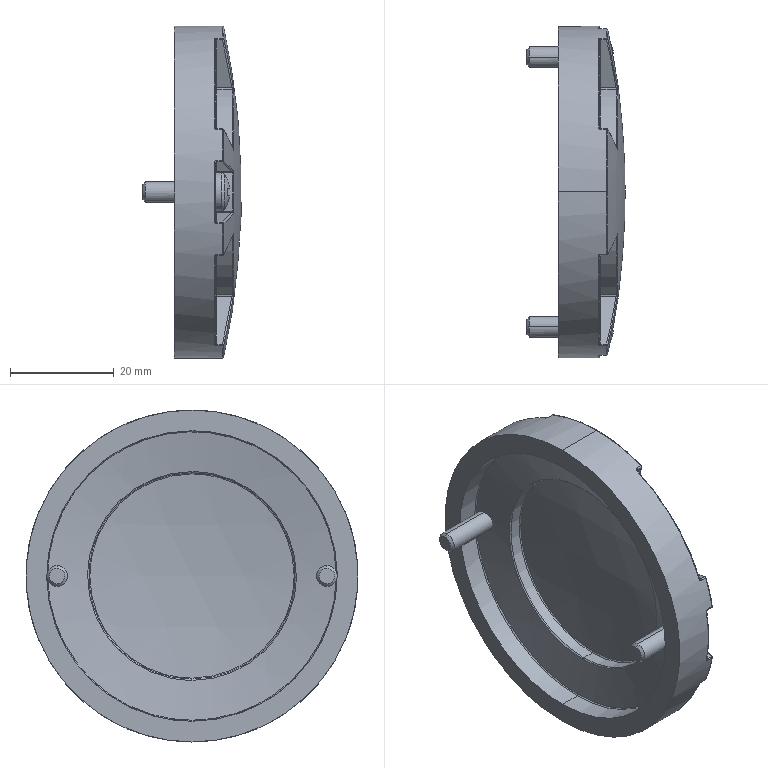Part | STEP file | 11-FCG-ZJ10011 | 1 solid | 257 faces | box 19 x 64 x 64 mm | volume 16815 mm3 | plane 69 | cylinder 65 | torus 46 | sphere 40 | spline 33 | cone 4 | commonest cylinder face diameters 0.5 x45 43 x6 4 x4 7.4 x4 39.8 x2 56 x2